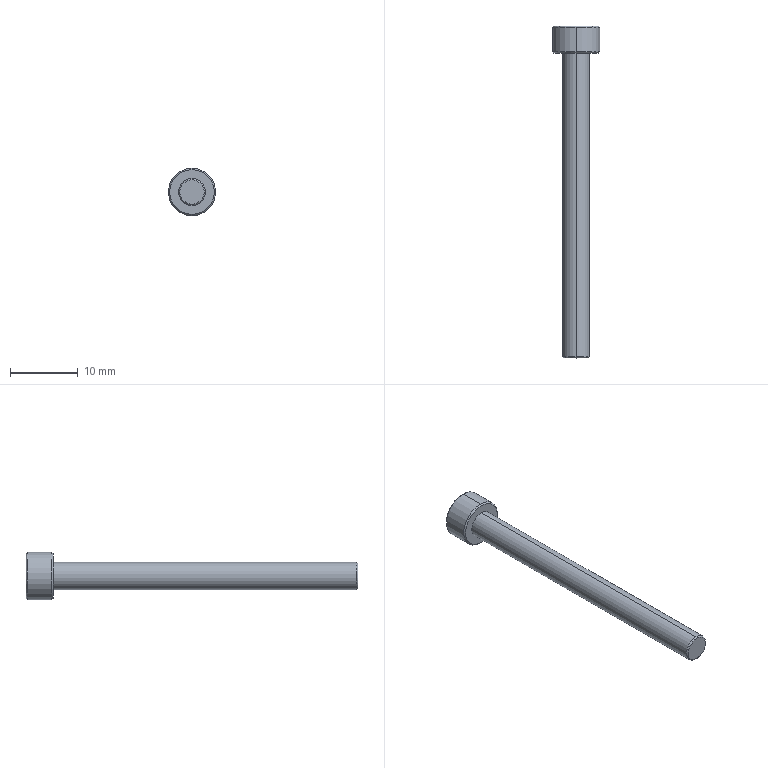Part | STEP file | Hex socket screw M4×45 | 1 solid | 33 faces | box 7 x 49 x 7 mm | volume 700.783 mm3 | cone 13 | plane 10 | spline 6 | cylinder 4 | commonest cylinder face diameters 4 x2 7 x2